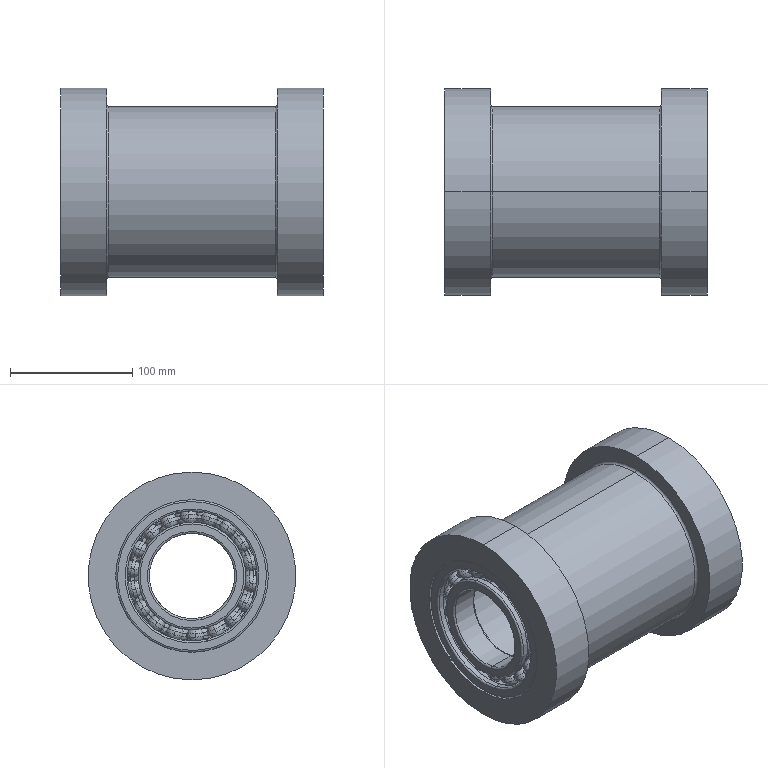Part | SolidWorks | features CompositeCurve 1 | 41 solids | 462 faces | box 215 x 170 x 170 mm | volume 2119651 mm3 | cylinder 176 | sphere 152 | plane 86 | torus 48 | commonest cylinder face diameters 94.75 x70 100.25 x70 88.333 x8 106.667 x8 125 x8 70 x4